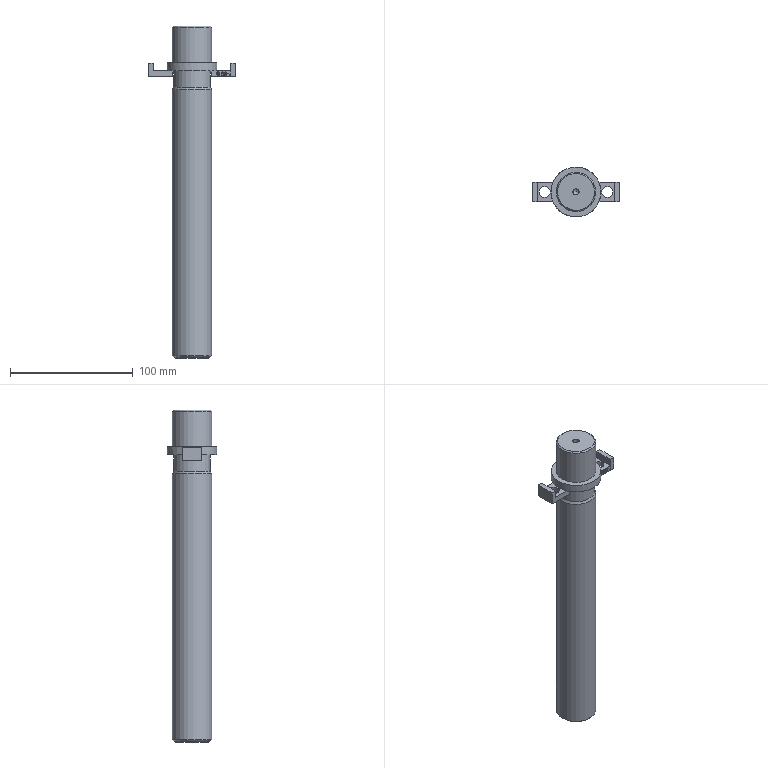Part | STEP file | lll_id4742_x_t | 1 solid | 122 faces | box 70.6 x 40.6 x 270 mm | volume 220646 mm3 | plane 70 | other 38 | cylinder 8 | cone 5 | torus 1 | commonest cylinder face diameters 9 x2 32 x2 5 x1 5.2 x1 30 x1 40.6 x1